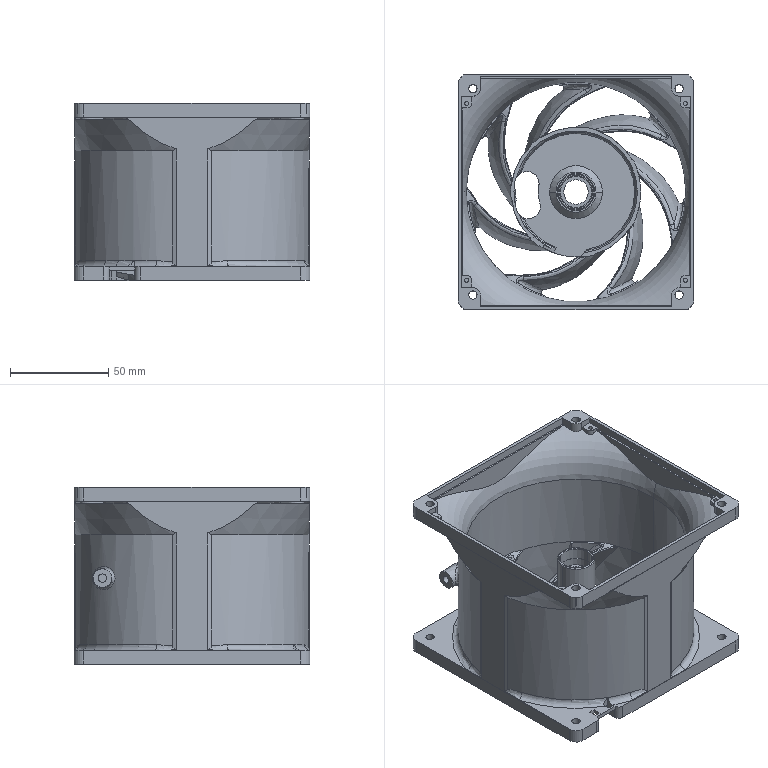CAM job | NX | 3-axis milling, drilling | part box 120 x 120 x 90.2 mm | stock box 138 x 138 x 95.2 mm
Tools:
number,name,description,diameter,corner_radius,flute_length,length,flutes
1,D12开粗刀,,12.0,0.0,50.0,60.0,2
2,D12-C,平底刀,12.0,0.0,58.0,65.0,4
3,D8开粗刀,,8.0,0.0,40.0,50.0,2
4,D6-C,平底刀,6.0,0.0,29.0,29.0,4
5,D4,平底刀,4.0,0.0,23.0,23.0,4
6,D8_J,平底刀,8.0,0.0,39.0,39.0,4
7,10R0.5,圆鼻刀,10.0,0.5,30.0,70.0,4
8,4R0.5,圆鼻刀,4.0,0.5,20.0,20.0,4
9,2R0.2-柄4,圆鼻刀,2.0,0.2,8.0,8.0,4
10,R3球刀,,6.0,3.0,30.0,35.0,2
11,R2,球刀,4.0,2.0,25.0,25.0,2
12,R1-柄4,球刀,2.0,1.0,0.0,15.0,2
13,倒角刀D4,,4.0,0.0,15.0,30.0,1
14,Z4.2,钻头,4.2,0.0,48.0,48.0,2
15,D10-C,平底刀,10.0,0.0,44.0,100.0,4
16,D10-J,平底刀,10.0,0.0,52.0,100.0,4
17,R4球刀,,8.0,4.0,40.0,60.0,2
18,R2球刀,,4.0,2.0,30.0,30.0,2
19,ZT2.1,,2.1,0.0,30.0,30.0,2
Operations:
program,operation,operation_type,tool,method,geometry_group,spindle_rpm,surface_speed,feed_per_tooth,feed_cut,feed_plunge,cut_length_mm,path_length_mm,cut_time_min,machine_time_min
干夹位,3D_ADAPTIVE_ROUGHING_COPY_1,SurfaceContour,D12开粗刀,AAA,M2,7500.0,282.743,0.3,4500.0,100.0,24654.501,31388.334,3.96,4.633
O01_1,2D斜开粗_COPY,PlanarMilling,D12-C,C0.3,M,7500.0,282.743,0.0167,500.0,100.0,346.88,458.23,0.6938,0.7049
O01_1,动态洗_COPY,SurfaceContour,D12-C,AAA,A,7500.0,282.743,0.15,4500.0,100.0,26929.669,29106.832,7.419,7.636
O01_1,动态洗_COPY_COPY,SurfaceContour,D12-C,AAA,A,7500.0,282.743,0.15,4500.0,100.0,22114.952,30474.453,4.202,5.038
O01_1,动态洗_COPY_COPY_COPY,SurfaceContour,D12-C,AAA,A,7500.0,282.743,0.15,4500.0,100.0,22232.361,31053.842,4.304,5.186
O01_1,动态洗_COPY_COPY_COPY_COPY,SurfaceContour,D12-C,AAA,A,7500.0,282.743,0.15,4500.0,100.0,22653.389,31409.1,4.418,5.293
O01_1,动态洗_COPY_COPY_COPY_COPY_COPY,SurfaceContour,D12-C,AAA,A,7500.0,282.743,0.15,4500.0,100.0,23231.721,32679.316,4.401,5.346
O13_1,QUICK_ROUGHING,SurfaceContour,D8开粗刀,METHOD,M,6800.0,6800.0,0.1838,2500.0,100.0,67614.28,90160.884,27.046,29.3
O13_1,QUICK_ROUGHING_COPY,SurfaceContour,D8开粗刀,METHOD,M,6800.0,6800.0,0.1838,2500.0,100.0,9873.451,13906.256,3.949,4.353
O13_1,QUICK_ROUGHING_COPY_COPY,SurfaceContour,D8开粗刀,METHOD,M,6800.0,6800.0,0.1838,2500.0,100.0,10963.345,14641.315,4.385,4.753
O13_1,QUICK_ROUGHING_COPY_COPY_COPY,SurfaceContour,D8开粗刀,METHOD,M,6800.0,6800.0,0.1838,2500.0,100.0,10945.982,14418.505,4.378,4.726
O13_1,QUICK_ROUGHING_COPY_COPY_COPY_COPY,SurfaceContour,D8开粗刀,METHOD,M,6800.0,6800.0,0.1838,2500.0,100.0,9278.254,12967.121,3.711,4.08
O12_1,QUICK_ROUGHING_COPY_1,SurfaceContour,D6-C,METHOD,M,6800.0,128.177,0.1103,3000.0,100.0,95641.146,116591.32,31.88,33.975
O12_1,QUICK_ROUGHING_COPY_1_COPY,SurfaceContour,D6-C,METHOD,M,6800.0,128.177,0.1103,3000.0,100.0,15890.511,23343.705,5.297,6.042
O12_1,QUICK_ROUGHING_COPY_1_COPY_COPY,SurfaceContour,D6-C,METHOD,M,6800.0,128.177,0.1103,3000.0,100.0,14214.032,20749.348,4.738,5.391
O12_1,QUICK_ROUGHING_COPY_1_COPY_COPY_COPY,SurfaceContour,D6-C,METHOD,M,6800.0,128.177,0.1103,3000.0,100.0,14778.132,21841.115,4.926,5.632
O01,型腔铣开粗铝料_COPY,CavityMilling,D4,METHOD,M,7500.0,94.248,0.0833,2500.0,100.0,16228.549,31123.021,6.491,7.981
O01_2,快捷洗平面_COPY_COPY_COPY_1_COPY,VolumeBased25DMillingOperation,D8_J,AAA,M,9500.0,238.761,0.0211,800.0,100.0,3747.837,4252.8,4.685,4.735
O01_2,快捷洗平面_COPY_COPY_COPY_1_COPY_COPY,VolumeBased25DMillingOperation,D8_J,AAA,M,9500.0,238.761,0.0211,800.0,100.0,1754.093,2178.392,2.193,2.235
O01_2,快捷洗平面_COPY_COPY_COPY_1_COPY_COPY_COPY,VolumeBased25DMillingOperation,D8_J,AAA,M,9500.0,238.761,0.0211,800.0,100.0,1754.093,2178.392,2.193,2.235
O01_2,快捷洗平面_COPY_COPY_COPY_1_COPY_COPY_COPY_COPY,VolumeBased25DMillingOperation,D8_J,AAA,M,9500.0,238.761,0.0211,800.0,100.0,1820.046,2515.066,2.275,2.345
O01_2,快捷洗平面_COPY_COPY_COPY_1_COPY_COPY_COPY_COPY_COPY,VolumeBased25DMillingOperation,D8_J,AAA,M,9500.0,238.761,0.0211,800.0,100.0,1860.334,2477.063,2.325,2.387
O03,等高精加工_COPY,ZLevelMilling,10R0.5,METHOD,M,6800.0,213.628,0.0735,2000.0,100.0,10448.016,10593.847,5.224,5.239
O03,等高精加工_COPY_COPY_1,ZLevelMilling,10R0.5,METHOD,M,6800.0,213.628,0.0735,2000.0,100.0,4063.179,8712.208,2.032,2.497
O04,等高精加工_COPY_COPY_1_COPY,ZLevelMilling,4R0.5,METHOD,M,7500.0,94.248,0.0667,2000.0,100.0,11982.316,13654.555,5.991,6.158
O04,快捷洗平面_COPY_COPY_COPY_1_COPY_COPY_COPY_COPY_COPY_COPY,VolumeBased25DMillingOperation,4R0.5,AAA,M,7500.0,94.248,0.0267,800.0,100.0,738.815,1896.13,0.9235,1.039
O05,等高精加工_COPY_COPY_1_COPY_COPY,ZLevelMilling,2R0.2-柄4,METHOD,M,8500.0,53.407,0.0441,1500.0,100.0,13964.493,24802.833,9.31,10.393
O02,AREA_MILL_COPY_COPY,SurfaceContour,R3球刀,AAA,M,8500.0,213.628,0.2059,3500.0,100.0,78197.386,79446.037,22.342,22.467
O02,AREA_MILL_COPY_COPY_COPY,SurfaceContour,R3球刀,AAA,M,8500.0,213.628,0.2059,3500.0,100.0,77854.332,79154.063,22.244,22.374
O02,AREA_MILL_COPY_COPY_COPY_COPY_1,SurfaceContour,R3球刀,AAA,M,8500.0,213.628,0.2059,3500.0,100.0,46216.96,47988.175,13.205,13.382
O02,AREA_MILL_COPY_COPY_COPY_COPY_1_COPY,SurfaceContour,R3球刀,AAA,M,8500.0,213.628,0.2059,3500.0,100.0,39723.116,44758.229,11.35,11.853
O02,AREA_MILL_COPY_COPY_COPY_COPY,SurfaceContour,R3球刀,AAA,M,8500.0,213.628,0.2059,3500.0,100.0,2695.445,3234.653,0.7701,0.824
O02,AREA_MILL_COPY_COPY_COPY_COPY_COPY,SurfaceContour,R3球刀,AAA,M,8500.0,213.628,0.2059,3500.0,100.0,2699.294,3129.055,0.7712,0.8142
O02,AREA_MILL_COPY_COPY_COPY_COPY_COPY_COPY,SurfaceContour,R3球刀,AAA,M,8500.0,213.628,0.2059,3500.0,100.0,2700.582,3226.388,0.7716,0.8242
O02_1,AREA_MILL_COPY_COPY_COPY_1,SurfaceContour,R3球刀,AAA,M,8500.0,213.628,0.2059,3500.0,100.0,94553.722,101601.754,27.015,27.72
O07,清根-参考刀具_COPY,SurfaceContour,R2,METHOD,M,7500.0,94.248,0.1,1500.0,100.0,22137.118,23862.204,14.758,14.931
O08,清根-参考刀具_COPY_COPY,SurfaceContour,R1-柄4,METHOD,M,8000.0,50.266,0.05,800.0,100.0,16306.667,17976.998,20.383,20.55
O02_1_1,钻孔打点_COPY_1,HoleDrilling,倒角刀D4,METHOD,M,2500.0,47.0,0.02,100.0,100.0,32.0,723.0,0.32,0.3891
O02_1_1,钻孔打点_COPY_1_COPY,HoleDrilling,倒角刀D4,METHOD,M,2500.0,47.0,0.02,100.0,100.0,8.0,102.0,0.08,0.0894
O01_2_1,G83钻孔_COPY_1,HoleDrilling,Z4.2,METHOD,M,1400.0,14.514,0.0179,50.0,0.0,389.331,1080.331,0.9409,1.01
O01_2_1,G83钻孔_COPY_1_COPY,HoleDrilling,Z4.2,METHOD,M,1400.0,14.514,0.0179,50.0,0.0,92.0,186.0,0.22,0.2294
O47,动态洗_COPY_COPY_1,SurfaceContour,D12-C,AAA,M1,7500.0,282.743,0.1167,3500.0,100.0,18335.278,18375.428,5.194,5.198
O21,动态洗_COPY_COPY_1_COPY,SurfaceContour,D12-C,AAA,M1,7500.0,282.743,0.1167,3500.0,100.0,58370.713,69528.907,16.033,17.149
O22,动态洗_COPY_COPY_1_COPY_COPY,SurfaceContour,D10-C,AAA,M1,7500.0,282.743,0.1167,3500.0,100.0,13161.423,24020.808,3.748,4.834
O23,等高精加工_COPY_COPY,ZLevelMilling,10R0.5,METHOD,M1,6800.0,213.628,0.1287,3500.0,100.0,165078.846,168903.695,47.165,47.548
O24,等高精加工_COPY_COPY_COPY,ZLevelMilling,4R0.5,METHOD,M1,8000.0,50.0,0.0938,1500.0,100.0,14836.467,19343.125,9.891,10.342
O25,等高精加工_COPY_COPY_COPY_COPY,ZLevelMilling,2R0.2-柄4,METHOD,M1,8000.0,50.0,0.0938,1500.0,100.0,11527.641,16404.12,7.685,8.173
O26,快捷洗平面_COPY_COPY_COPY_1_COPY_COPY_1,VolumeBased25DMillingOperation,D8_J,AAA,M1,9500.0,238.761,0.0132,500.0,100.0,2008.007,2978.302,4.016,4.113
O27,等高精加工_COPY_COPY_2,ZLevelMilling,10R0.5,METHOD,M1,5200.0,163.363,0.0721,1500.0,100.0,853.287,1028.531,0.5689,0.5864
O27,等高精加工_COPY_COPY_2_COPY,ZLevelMilling,10R0.5,METHOD,M1,5200.0,163.363,0.0721,1500.0,100.0,3000.167,3175.405,2,2.018
O29,等高精加工_COPY_COPY_2_COPY_COPY,ZLevelMilling,10R0.5,METHOD,M1,6800.0,213.628,0.1103,3000.0,100.0,22524.975,24278.4,7.508,7.684
O28,快捷洗平面_COPY_COPY_COPY_1_COPY_COPY_2,VolumeBased25DMillingOperation,D10-J,AAA,M1,9500.0,298.451,0.0316,1200.0,100.0,1370.579,2309.805,1.142,1.236
O28,快捷洗平面_COPY_COPY_COPY_1_COPY_COPY_2_COPY,VolumeBased25DMillingOperation,D10-J,AAA,M1,9500.0,298.451,0.0316,1200.0,100.0,837.895,1621.856,0.6982,0.7766
O41,AREA_MILL_COPY_COPY_COPY_2,SurfaceContour,R4球刀,AAA,M1,6800.0,170.903,0.1838,2500.0,100.0,39632.256,41198.88,15.853,16.01
O44,FIXED_AXIS_GUIDING_CURVES_COPY,SurfaceContour,R3球刀,AAA,M1,7500.0,141.372,0.2,3000.0,100.0,10121.085,10400.226,3.374,3.402
O44,FIXED_AXIS_GUIDING_CURVES_COPY_INSTANCE,SurfaceContour,R3球刀,AAA,M1,7500.0,141.372,0.2,3000.0,100.0,10121.085,10400.226,3.374,3.402
O44,FIXED_AXIS_GUIDING_CURVES_COPY_INSTANCE_1,SurfaceContour,R3球刀,AAA,M1,7500.0,141.372,0.2,3000.0,100.0,10121.085,10400.226,3.374,3.402
O44,FIXED_AXIS_GUIDING_CURVES_COPY_INSTANCE_2,SurfaceContour,R3球刀,AAA,M1,7500.0,141.372,0.2,3000.0,100.0,10121.085,10400.226,3.374,3.402
O44,FIXED_AXIS_GUIDING_CURVES_COPY_INSTANCE_3,SurfaceContour,R3球刀,AAA,M1,7500.0,141.372,0.2,3000.0,100.0,10121.085,10400.226,3.374,3.402
O44,FIXED_AXIS_GUIDING_CURVES_COPY_INSTANCE_4,SurfaceContour,R3球刀,AAA,M1,7500.0,141.372,0.2,3000.0,100.0,10121.085,10400.226,3.374,3.402
O44,FIXED_AXIS_GUIDING_CURVES_COPY_INSTANCE_5,SurfaceContour,R3球刀,AAA,M1,7500.0,141.372,0.2,3000.0,100.0,10121.085,10400.226,3.374,3.402
O43,FIXED_AXIS_GUIDING_CURVES,SurfaceContour,R2球刀,AAA,M1,8000.0,100.531,0.1562,2500.0,100.0,17260.801,18017.841,6.904,6.98
O43,FIXED_AXIS_GUIDING_CURVES_INSTANCE,SurfaceContour,R2球刀,AAA,M1,8000.0,100.531,0.1562,2500.0,100.0,17260.801,18017.841,6.904,6.98
O43,FIXED_AXIS_GUIDING_CURVES_INSTANCE_1,SurfaceContour,R2球刀,AAA,M1,8000.0,100.531,0.1562,2500.0,100.0,17260.801,18017.841,6.904,6.98
O43,FIXED_AXIS_GUIDING_CURVES_INSTANCE_2,SurfaceContour,R2球刀,AAA,M1,8000.0,100.531,0.1562,2500.0,100.0,17260.801,18017.841,6.904,6.98
O43,FIXED_AXIS_GUIDING_CURVES_INSTANCE_3,SurfaceContour,R2球刀,AAA,M1,8000.0,100.531,0.1562,2500.0,100.0,17260.801,18017.841,6.904,6.98
O43,FIXED_AXIS_GUIDING_CURVES_INSTANCE_4,SurfaceContour,R2球刀,AAA,M1,8000.0,100.531,0.1562,2500.0,100.0,17260.801,18017.841,6.904,6.98
O43,FIXED_AXIS_GUIDING_CURVES_COPY_1,SurfaceContour,R2球刀,AAA,M1,8000.0,100.531,0.1562,2500.0,100.0,17113.918,17372.984,6.846,6.872
O45,钻孔打点_COPY_1_COPY_1,HoleDrilling,倒角刀D4,METHOD,M1,2500.0,47.0,0.02,100.0,100.0,64.0,1165.169,0.64,0.7501
O02_1_1_COPY,G83钻孔_COPY_1_COPY_1,HoleDrilling,Z4.2,METHOD,M1,1400.0,14.514,0.0179,50.0,0.0,480.378,1171.378,1.021,1.09
O46,G83钻孔_COPY_1_COPY_1_COPY,HoleDrilling,ZT2.1,METHOD,M1,1400.0,14.514,0.0179,50.0,0.0,198.618,866.018,0.6505,0.7172